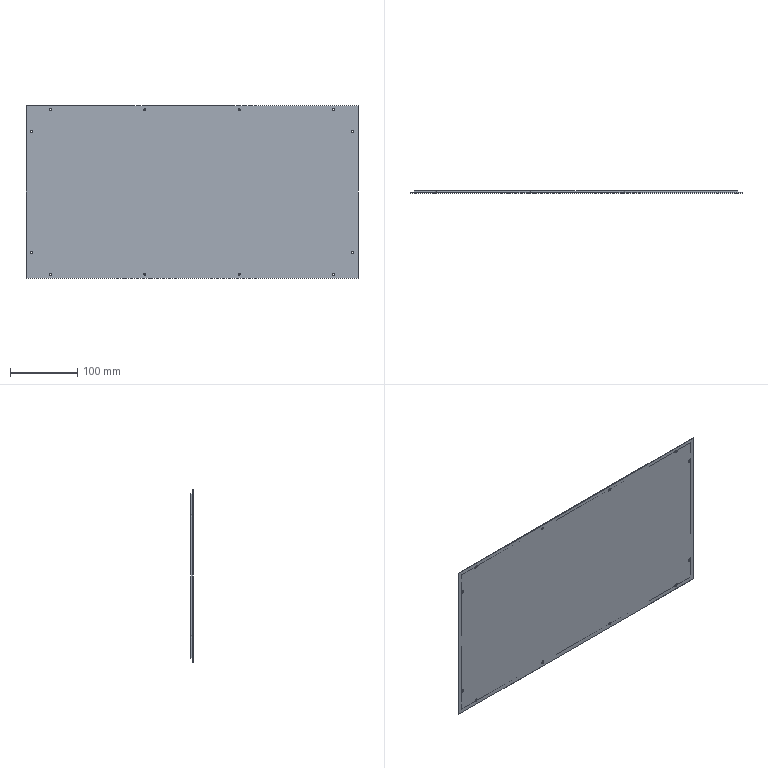Part | SolidWorks | features ICE 4, MirrorPattern 2, Extrusion 1 | 1 solid | 71 faces | box 493 x 3 x 256.3 mm | volume 360860 mm3 | cylinder 48 | plane 23 | commonest cylinder face diameters 3 x24 6 x24